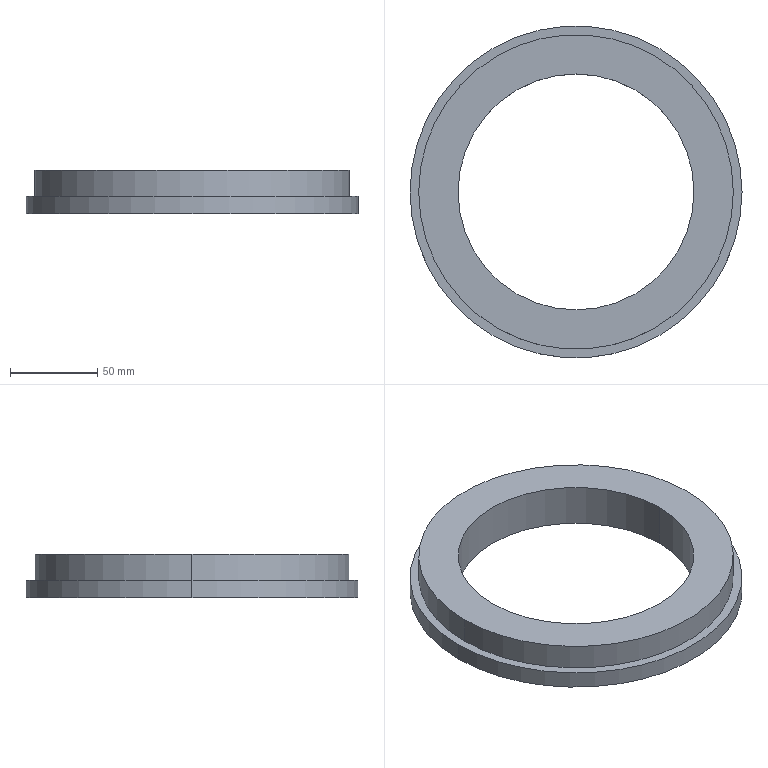Part | SolidWorks | features 3DProfileFeature 1, Extrusion 1, HoleWzd 1, ICE 1 | 1 solid | 33 faces | box 190 x 190 x 25 mm | volume 301982 mm3 | cylinder 18 | cone 12 | plane 3 | commonest cylinder face diameters 10.2 x12 135 x2 180 x2 190 x2
STEP:
#1=CARTESIAN_POINT('',(5.1,80.5,10.));
#2=VERTEX_POINT('',#1);
#3=CARTESIAN_POINT('',(-5.1,80.5,10.));
#4=VERTEX_POINT('',#3);
#5=CARTESIAN_POINT('',(0.,80.5,10.));
#6=DIRECTION('',(0.,0.,-1.));
#7=DIRECTION('',(-1.,0.,0.));
#8=AXIS2_PLACEMENT_3D('',#5,#6,#7);
#9=CIRCLE('',#8,5.1);
#10=EDGE_CURVE('',#2,#4,#9,.T.);
#11=ORIENTED_EDGE('',*,*,#10,.F.);
#12=CARTESIAN_POINT('',(5.1,80.5,0.));
#13=VERTEX_POINT('',#12);
#14=CARTESIAN_POINT('',(5.1,80.5,0.));
#15=DIRECTION('',(0.,0.,-1.));
#16=VECTOR('',#15,1000.);
#17=LINE('',#14,#16);
#18=EDGE_CURVE('',#2,#13,#17,.T.);
#19=ORIENTED_EDGE('',*,*,#18,.T.);
#20=CARTESIAN_POINT('',(-5.1,80.5,0.));
#21=VERTEX_POINT('',#20);
#22=CARTESIAN_POINT('',(0.,80.5,0.));
#23=DIRECTION('',(0.,0.,-1.));
#24=DIRECTION('',(-1.,0.,0.));
#25=AXIS2_PLACEMENT_3D('',#22,#23,#24);
#26=CIRCLE('',#25,5.1);
#27=EDGE_CURVE('',#13,#21,#26,.T.);
#28=ORIENTED_EDGE('',*,*,#27,.T.);
#29=CARTESIAN_POINT('',(-5.1,80.5,0.));
#30=DIRECTION('',(0.,0.,-1.));
#31=VECTOR('',#30,1000.);
#32=LINE('',#29,#31);
#33=EDGE_CURVE('',#4,#21,#32,.T.);
#34=ORIENTED_EDGE('',*,*,#33,.F.);
#35=EDGE_LOOP('',(#11,#19,#28,#34));
#36=FACE_OUTER_BOUND('',#35,.T.);
#37=CARTESIAN_POINT('',(0.,80.5,0.));
#38=DIRECTION('',(0.,0.,-1.));
#39=DIRECTION('',(-1.,0.,0.));
#40=AXIS2_PLACEMENT_3D('',#37,#38,#39);
#41=CYLINDRICAL_SURFACE('',#40,5.1);
#42=ADVANCED_FACE('',(#36),#41,.F.);
#43=CARTESIAN_POINT('',(0.,80.5,13.064));
#44=VERTEX_POINT('',#43);
#45=CARTESIAN_POINT('',(-5.1,80.5,10.));
#46=DIRECTION('',(-0.8572,0.,-0.515));
#47=VECTOR('',#46,1000.);
#48=LINE('',#45,#47);
#49=EDGE_CURVE('',#44,#4,#48,.T.);
#50=ORIENTED_EDGE('',*,*,#49,.F.);
#51=CARTESIAN_POINT('',(5.1,80.5,10.));
#52=DIRECTION('',(0.8572,0.,-0.515));
#53=VECTOR('',#52,1000.);
#54=LINE('',#51,#53);
#55=EDGE_CURVE('',#44,#2,#54,.T.);
#56=ORIENTED_EDGE('',*,*,#55,.T.);
#57=ORIENTED_EDGE('',*,*,#10,.T.);
#58=EDGE_LOOP('',(#50,#56,#57));
#59=FACE_OUTER_BOUND('',#58,.T.);
#60=CARTESIAN_POINT('',(0.,80.5,10.));
#61=DIRECTION('',(0.,0.,-1.));
#62=DIRECTION('',(-1.,0.,0.));
#63=AXIS2_PLACEMENT_3D('',#60,#61,#62);
#64=CONICAL_SURFACE('',#63,5.1,1.03);
#65=ADVANCED_FACE('',(#59),#64,.F.);
#66=CARTESIAN_POINT('',(74.815,40.25,10.));
#67=VERTEX_POINT('',#66);
#68=CARTESIAN_POINT('',(64.615,40.25,10.));
#69=VERTEX_POINT('',#68);
#70=CARTESIAN_POINT('',(69.715,40.25,10.));
#71=DIRECTION('',(0.,0.,-1.));
#72=DIRECTION('',(-1.,0.,0.));
#73=AXIS2_PLACEMENT_3D('',#70,#71,#72);
#74=CIRCLE('',#73,5.1);
#75=EDGE_CURVE('',#67,#69,#74,.T.);
#76=ORIENTED_EDGE('',*,*,#75,.F.);
#77=CARTESIAN_POINT('',(74.815,40.25,0.));
#78=VERTEX_POINT('',#77);
#79=CARTESIAN_POINT('',(74.815,40.25,0.));
#80=DIRECTION('',(0.,0.,-1.));
#81=VECTOR('',#80,1000.);
#82=LINE('',#79,#81);
#83=EDGE_CURVE('',#67,#78,#82,.T.);
#84=ORIENTED_EDGE('',*,*,#83,.T.);
#85=CARTESIAN_POINT('',(64.615,40.25,0.));
#86=VERTEX_POINT('',#85);
#87=CARTESIAN_POINT('',(69.715,40.25,0.));
#88=DIRECTION('',(0.,0.,-1.));
#89=DIRECTION('',(-1.,0.,0.));
#90=AXIS2_PLACEMENT_3D('',#87,#88,#89);
#91=CIRCLE('',#90,5.1);
#92=EDGE_CURVE('',#78,#86,#91,.T.);
#93=ORIENTED_EDGE('',*,*,#92,.T.);
#94=CARTESIAN_POINT('',(64.615,40.25,0.));
#95=DIRECTION('',(0.,0.,-1.));
#96=VECTOR('',#95,1000.);
#97=LINE('',#94,#96);
#98=EDGE_CURVE('',#69,#86,#97,.T.);
#99=ORIENTED_EDGE('',*,*,#98,.F.);
#100=EDGE_LOOP('',(#76,#84,#93,#99));
#101=FACE_OUTER_BOUND('',#100,.T.);
#102=CARTESIAN_POINT('',(69.715,40.25,0.));
#103=DIRECTION('',(0.,0.,-1.));
#104=DIRECTION('',(-1.,0.,0.));
#105=AXIS2_PLACEMENT_3D('',#102,#103,#104);
#106=CYLINDRICAL_SURFACE('',#105,5.1);
#107=ADVANCED_FACE('',(#101),#106,.F.);
#108=CARTESIAN_POINT('',(69.715,40.25,13.064));
#109=VERTEX_POINT('',#108);
#110=CARTESIAN_POINT('',(64.615,40.25,10.));
#111=DIRECTION('',(-0.8572,0.,-0.515));
#112=VECTOR('',#111,1000.);
#113=LINE('',#110,#112);
#114=EDGE_CURVE('',#109,#69,#113,.T.);
#115=ORIENTED_EDGE('',*,*,#114,.F.);
#116=CARTESIAN_POINT('',(74.815,40.25,10.));
#117=DIRECTION('',(0.8572,0.,-0.515));
#118=VECTOR('',#117,1000.);
#119=LINE('',#116,#118);
#120=EDGE_CURVE('',#109,#67,#119,.T.);
#121=ORIENTED_EDGE('',*,*,#120,.T.);
#122=ORIENTED_EDGE('',*,*,#75,.T.);
#123=EDGE_LOOP('',(#115,#121,#122));
#124=FACE_OUTER_BOUND('',#123,.T.);
#125=CARTESIAN_POINT('',(69.715,40.25,10.));
#126=DIRECTION('',(0.,0.,-1.));
#127=DIRECTION('',(-1.,0.,0.));
#128=AXIS2_PLACEMENT_3D('',#125,#126,#127);
#129=CONICAL_SURFACE('',#128,5.1,1.03);
#130=ADVANCED_FACE('',(#124),#129,.F.);
#131=CARTESIAN_POINT('',(74.815,-40.25,10.));
#132=VERTEX_POINT('',#131);
#133=CARTESIAN_POINT('',(64.615,-40.25,10.));
#134=VERTEX_POINT('',#133);
#135=CARTESIAN_POINT('',(69.715,-40.25,10.));
#136=DIRECTION('',(0.,0.,-1.));
#137=DIRECTION('',(-1.,0.,0.));
#138=AXIS2_PLACEMENT_3D('',#135,#136,#137);
#139=CIRCLE('',#138,5.1);
#140=EDGE_CURVE('',#132,#134,#139,.T.);
#141=ORIENTED_EDGE('',*,*,#140,.F.);
#142=CARTESIAN_POINT('',(74.815,-40.25,0.));
#143=VERTEX_POINT('',#142);
#144=CARTESIAN_POINT('',(74.815,-40.25,0.));
#145=DIRECTION('',(0.,0.,-1.));
#146=VECTOR('',#145,1000.);
#147=LINE('',#144,#146);
#148=EDGE_CURVE('',#132,#143,#147,.T.);
#149=ORIENTED_EDGE('',*,*,#148,.T.);
#150=CARTESIAN_POINT('',(64.615,-40.25,0.));
#151=VERTEX_POINT('',#150);
#152=CARTESIAN_POINT('',(69.715,-40.25,0.));
#153=DIRECTION('',(0.,0.,-1.));
#154=DIRECTION('',(-1.,0.,0.));
#155=AXIS2_PLACEMENT_3D('',#152,#153,#154);
#156=CIRCLE('',#155,5.1);
#157=EDGE_CURVE('',#143,#151,#156,.T.);
#158=ORIENTED_EDGE('',*,*,#157,.T.);
#159=CARTESIAN_POINT('',(64.615,-40.25,0.));
#160=DIRECTION('',(0.,0.,-1.));
#161=VECTOR('',#160,1000.);
#162=LINE('',#159,#161);
#163=EDGE_CURVE('',#134,#151,#162,.T.);
#164=ORIENTED_EDGE('',*,*,#163,.F.);
#165=EDGE_LOOP('',(#141,#149,#158,#164));
#166=FACE_OUTER_BOUND('',#165,.T.);
#167=CARTESIAN_POINT('',(69.715,-40.25,0.));
#168=DIRECTION('',(0.,0.,-1.));
#169=DIRECTION('',(-1.,0.,0.));
#170=AXIS2_PLACEMENT_3D('',#167,#168,#169);
#171=CYLINDRICAL_SURFACE('',#170,5.1);
#172=ADVANCED_FACE('',(#166),#171,.F.);
#173=CARTESIAN_POINT('',(69.715,-40.25,13.064));
#174=VERTEX_POINT('',#173);
#175=CARTESIAN_POINT('',(64.615,-40.25,10.));
#176=DIRECTION('',(-0.8572,0.,-0.515));
#177=VECTOR('',#176,1000.);
#178=LINE('',#175,#177);
#179=EDGE_CURVE('',#174,#134,#178,.T.);
#180=ORIENTED_EDGE('',*,*,#179,.F.);
#181=CARTESIAN_POINT('',(74.815,-40.25,10.));
#182=DIRECTION('',(0.8572,0.,-0.515));
#183=VECTOR('',#182,1000.);
#184=LINE('',#181,#183);
#185=EDGE_CURVE('',#174,#132,#184,.T.);
#186=ORIENTED_EDGE('',*,*,#185,.T.);
#187=ORIENTED_EDGE('',*,*,#140,.T.);
#188=EDGE_LOOP('',(#180,#186,#187));
#189=FACE_OUTER_BOUND('',#188,.T.);
#190=CARTESIAN_POINT('',(69.715,-40.25,10.));
#191=DIRECTION('',(0.,0.,-1.));
#192=DIRECTION('',(-1.,0.,0.));
#193=AXIS2_PLACEMENT_3D('',#190,#191,#192);
#194=CONICAL_SURFACE('',#193,5.1,1.03);
#195=ADVANCED_FACE('',(#189),#194,.F.);
#196=CARTESIAN_POINT('',(5.1,-80.5,10.));
#197=VERTEX_POINT('',#196);
#198=CARTESIAN_POINT('',(-5.1,-80.5,10.));
#199=VERTEX_POINT('',#198);
#200=CARTESIAN_POINT('',(0.,-80.5,10.));
#201=DIRECTION('',(0.,0.,-1.));
#202=DIRECTION('',(-1.,0.,0.));
#203=AXIS2_PLACEMENT_3D('',#200,#201,#202);
#204=CIRCLE('',#203,5.1);
#205=EDGE_CURVE('',#197,#199,#204,.T.);
#206=ORIENTED_EDGE('',*,*,#205,.F.);
#207=CARTESIAN_POINT('',(5.1,-80.5,0.));
#208=VERTEX_POINT('',#207);
#209=CARTESIAN_POINT('',(5.1,-80.5,0.));
#210=DIRECTION('',(0.,0.,-1.));
#211=VECTOR('',#210,1000.);
#212=LINE('',#209,#211);
#213=EDGE_CURVE('',#197,#208,#212,.T.);
#214=ORIENTED_EDGE('',*,*,#213,.T.);
#215=CARTESIAN_POINT('',(-5.1,-80.5,0.));
#216=VERTEX_POINT('',#215);
#217=CARTESIAN_POINT('',(0.,-80.5,0.));
#218=DIRECTION('',(0.,0.,-1.));
#219=DIRECTION('',(-1.,0.,0.));
#220=AXIS2_PLACEMENT_3D('',#217,#218,#219);
#221=CIRCLE('',#220,5.1);
#222=EDGE_CURVE('',#208,#216,#221,.T.);
#223=ORIENTED_EDGE('',*,*,#222,.T.);
#224=CARTESIAN_POINT('',(-5.1,-80.5,0.));
#225=DIRECTION('',(0.,0.,-1.));
#226=VECTOR('',#225,1000.);
#227=LINE('',#224,#226);
#228=EDGE_CURVE('',#199,#216,#227,.T.);
#229=ORIENTED_EDGE('',*,*,#228,.F.);
#230=EDGE_LOOP('',(#206,#214,#223,#229));
#231=FACE_OUTER_BOUND('',#230,.T.);
#232=CARTESIAN_POINT('',(0.,-80.5,0.));
#233=DIRECTION('',(0.,0.,-1.));
#234=DIRECTION('',(-1.,0.,0.));
#235=AXIS2_PLACEMENT_3D('',#232,#233,#234);
#236=CYLINDRICAL_SURFACE('',#235,5.1);
#237=ADVANCED_FACE('',(#231),#236,.F.);
#238=CARTESIAN_POINT('',(0.,-80.5,13.064));
#239=VERTEX_POINT('',#238);
#240=CARTESIAN_POINT('',(-5.1,-80.5,10.));
#241=DIRECTION('',(-0.8572,0.,-0.515));
#242=VECTOR('',#241,1000.);
#243=LINE('',#240,#242);
#244=EDGE_CURVE('',#239,#199,#243,.T.);
#245=ORIENTED_EDGE('',*,*,#244,.F.);
#246=CARTESIAN_POINT('',(5.1,-80.5,10.));
#247=DIRECTION('',(0.8572,0.,-0.515));
#248=VECTOR('',#247,1000.);
#249=LINE('',#246,#248);
#250=EDGE_CURVE('',#239,#197,#249,.T.);
#251=ORIENTED_EDGE('',*,*,#250,.T.);
#252=ORIENTED_EDGE('',*,*,#205,.T.);
#253=EDGE_LOOP('',(#245,#251,#252));
#254=FACE_OUTER_BOUND('',#253,.T.);
#255=CARTESIAN_POINT('',(0.,-80.5,10.));
#256=DIRECTION('',(0.,0.,-1.));
#257=DIRECTION('',(-1.,0.,0.));
#258=AXIS2_PLACEMENT_3D('',#255,#256,#257);
#259=CONICAL_SURFACE('',#258,5.1,1.03);
#260=ADVANCED_FACE('',(#254),#259,.F.);
#261=CARTESIAN_POINT('',(-64.615,-40.25,10.));
#262=VERTEX_POINT('',#261);
#263=CARTESIAN_POINT('',(-74.815,-40.25,10.));
#264=VERTEX_POINT('',#263);
#265=CARTESIAN_POINT('',(-69.715,-40.25,10.));
#266=DIRECTION('',(0.,0.,-1.));
#267=DIRECTION('',(-1.,0.,0.));
#268=AXIS2_PLACEMENT_3D('',#265,#266,#267);
#269=CIRCLE('',#268,5.1);
#270=EDGE_CURVE('',#262,#264,#269,.T.);
#271=ORIENTED_EDGE('',*,*,#270,.F.);
#272=CARTESIAN_POINT('',(-64.615,-40.25,0.));
#273=VERTEX_POINT('',#272);
#274=CARTESIAN_POINT('',(-64.615,-40.25,0.));
#275=DIRECTION('',(0.,0.,-1.));
#276=VECTOR('',#275,1000.);
#277=LINE('',#274,#276);
#278=EDGE_CURVE('',#262,#273,#277,.T.);
#279=ORIENTED_EDGE('',*,*,#278,.T.);
#280=CARTESIAN_POINT('',(-74.815,-40.25,0.));
#281=VERTEX_POINT('',#280);
#282=CARTESIAN_POINT('',(-69.715,-40.25,0.));
#283=DIRECTION('',(0.,0.,-1.));
#284=DIRECTION('',(-1.,0.,0.));
#285=AXIS2_PLACEMENT_3D('',#282,#283,#284);
#286=CIRCLE('',#285,5.1);
#287=EDGE_CURVE('',#273,#281,#286,.T.);
#288=ORIENTED_EDGE('',*,*,#287,.T.);
#289=CARTESIAN_POINT('',(-74.815,-40.25,0.));
#290=DIRECTION('',(0.,0.,-1.));
#291=VECTOR('',#290,1000.);
#292=LINE('',#289,#291);
#293=EDGE_CURVE('',#264,#281,#292,.T.);
#294=ORIENTED_EDGE('',*,*,#293,.F.);
#295=EDGE_LOOP('',(#271,#279,#288,#294));
#296=FACE_OUTER_BOUND('',#295,.T.);
#297=CARTESIAN_POINT('',(-69.715,-40.25,0.));
#298=DIRECTION('',(0.,0.,-1.));
#299=DIRECTION('',(-1.,0.,0.));
#300=AXIS2_PLACEMENT_3D('',#297,#298,#299);
#301=CYLINDRICAL_SURFACE('',#300,5.1);
#302=ADVANCED_FACE('',(#296),#301,.F.);
#303=CARTESIAN_POINT('',(-69.715,-40.25,13.064));
#304=VERTEX_POINT('',#303);
#305=CARTESIAN_POINT('',(-74.815,-40.25,10.));
#306=DIRECTION('',(-0.8572,0.,-0.515));
#307=VECTOR('',#306,1000.);
#308=LINE('',#305,#307);
#309=EDGE_CURVE('',#304,#264,#308,.T.);
#310=ORIENTED_EDGE('',*,*,#309,.F.);
#311=CARTESIAN_POINT('',(-64.615,-40.25,10.));
#312=DIRECTION('',(0.8572,0.,-0.515));
#313=VECTOR('',#312,1000.);
#314=LINE('',#311,#313);
#315=EDGE_CURVE('',#304,#262,#314,.T.);
#316=ORIENTED_EDGE('',*,*,#315,.T.);
#317=ORIENTED_EDGE('',*,*,#270,.T.);
#318=EDGE_LOOP('',(#310,#316,#317));
#319=FACE_OUTER_BOUND('',#318,.T.);
#320=CARTESIAN_POINT('',(-69.715,-40.25,10.));
#321=DIRECTION('',(0.,0.,-1.));
#322=DIRECTION('',(-1.,0.,0.));
#323=AXIS2_PLACEMENT_3D('',#320,#321,#322);
#324=CONICAL_SURFACE('',#323,5.1,1.03);
#325=ADVANCED_FACE('',(#319),#324,.F.);
#326=CARTESIAN_POINT('',(-64.615,40.25,10.));
#327=VERTEX_POINT('',#326);
#328=CARTESIAN_POINT('',(-74.815,40.25,10.));
#329=VERTEX_POINT('',#328);
#330=CARTESIAN_POINT('',(-69.715,40.25,10.));
#331=DIRECTION('',(0.,0.,-1.));
#332=DIRECTION('',(-1.,0.,0.));
#333=AXIS2_PLACEMENT_3D('',#330,#331,#332);
#334=CIRCLE('',#333,5.1);
#335=EDGE_CURVE('',#327,#329,#334,.T.);
#336=ORIENTED_EDGE('',*,*,#335,.F.);
#337=CARTESIAN_POINT('',(-64.615,40.25,0.));
#338=VERTEX_POINT('',#337);
#339=CARTESIAN_POINT('',(-64.615,40.25,0.));
#340=DIRECTION('',(0.,0.,-1.));
#341=VECTOR('',#340,1000.);
#342=LINE('',#339,#341);
#343=EDGE_CURVE('',#327,#338,#342,.T.);
#344=ORIENTED_EDGE('',*,*,#343,.T.);
#345=CARTESIAN_POINT('',(-74.815,40.25,0.));
#346=VERTEX_POINT('',#345);
#347=CARTESIAN_POINT('',(-69.715,40.25,0.));
#348=DIRECTION('',(0.,0.,-1.));
#349=DIRECTION('',(-1.,0.,0.));
#350=AXIS2_PLACEMENT_3D('',#347,#348,#349);
#351=CIRCLE('',#350,5.1);
#352=EDGE_CURVE('',#338,#346,#351,.T.);
#353=ORIENTED_EDGE('',*,*,#352,.T.);
#354=CARTESIAN_POINT('',(-74.815,40.25,0.));
#355=DIRECTION('',(0.,0.,-1.));
#356=VECTOR('',#355,1000.);
#357=LINE('',#354,#356);
#358=EDGE_CURVE('',#329,#346,#357,.T.);
#359=ORIENTED_EDGE('',*,*,#358,.F.);
#360=EDGE_LOOP('',(#336,#344,#353,#359));
#361=FACE_OUTER_BOUND('',#360,.T.);
#362=CARTESIAN_POINT('',(-69.715,40.25,0.));
#363=DIRECTION('',(0.,0.,-1.));
#364=DIRECTION('',(-1.,0.,0.));
#365=AXIS2_PLACEMENT_3D('',#362,#363,#364);
#366=CYLINDRICAL_SURFACE('',#365,5.1);
#367=ADVANCED_FACE('',(#361),#366,.F.);
#368=CARTESIAN_POINT('',(-69.715,40.25,13.064));
#369=VERTEX_POINT('',#368);
#370=CARTESIAN_POINT('',(-74.815,40.25,10.));
#371=DIRECTION('',(-0.8572,0.,-0.515));
#372=VECTOR('',#371,1000.);
#373=LINE('',#370,#372);
#374=EDGE_CURVE('',#369,#329,#373,.T.);
#375=ORIENTED_EDGE('',*,*,#374,.F.);
#376=CARTESIAN_POINT('',(-64.615,40.25,10.));
#377=DIRECTION('',(0.8572,0.,-0.515));
#378=VECTOR('',#377,1000.);
#379=LINE('',#376,#378);
#380=EDGE_CURVE('',#369,#327,#379,.T.);
#381=ORIENTED_EDGE('',*,*,#380,.T.);
#382=ORIENTED_EDGE('',*,*,#335,.T.);
#383=EDGE_LOOP('',(#375,#381,#382));
#384=FACE_OUTER_BOUND('',#383,.T.);
#385=CARTESIAN_POINT('',(-69.715,40.25,10.));
#386=DIRECTION('',(0.,0.,-1.));
#387=DIRECTION('',(-1.,0.,0.));
#388=AXIS2_PLACEMENT_3D('',#385,#386,#387);
#389=CONICAL_SURFACE('',#388,5.1,1.03);
#390=ADVANCED_FACE('',(#384),#389,.F.);
#391=CARTESIAN_POINT('',(90.,0.,25.));
#392=VERTEX_POINT('',#391);
#393=CARTESIAN_POINT('',(-90.,0.,25.));
#394=VERTEX_POINT('',#393);
#395=CARTESIAN_POINT('',(0.,0.,25.));
#396=DIRECTION('',(0.,0.,1.));
#397=DIRECTION('',(1.,0.,0.));
#398=AXIS2_PLACEMENT_3D('',#395,#396,#397);
#399=CIRCLE('',#398,90.);
#400=EDGE_CURVE('',#392,#394,#399,.T.);
#401=ORIENTED_EDGE('',*,*,#400,.F.);
#402=CARTESIAN_POINT('',(90.,0.,10.));
#403=VERTEX_POINT('',#402);
#404=CARTESIAN_POINT('',(90.,0.,25.));
#405=DIRECTION('',(0.,0.,-1.));
#406=VECTOR('',#405,1000.);
#407=LINE('',#404,#406);
#408=EDGE_CURVE('',#392,#403,#407,.T.);
#409=ORIENTED_EDGE('',*,*,#408,.T.);
#410=CARTESIAN_POINT('',(-90.,0.,10.));
#411=VERTEX_POINT('',#410);
#412=CARTESIAN_POINT('',(0.,0.,10.));
#413=DIRECTION('',(0.,0.,1.));
#414=DIRECTION('',(1.,0.,0.));
#415=AXIS2_PLACEMENT_3D('',#412,#413,#414);
#416=CIRCLE('',#415,90.);
#417=EDGE_CURVE('',#403,#411,#416,.T.);
#418=ORIENTED_EDGE('',*,*,#417,.T.);
#419=CARTESIAN_POINT('',(-90.,0.,25.));
#420=DIRECTION('',(0.,0.,-1.));
#421=VECTOR('',#420,1000.);
#422=LINE('',#419,#421);
#423=EDGE_CURVE('',#394,#411,#422,.T.);
#424=ORIENTED_EDGE('',*,*,#423,.F.);
#425=EDGE_LOOP('',(#401,#409,#418,#424));
#426=FACE_OUTER_BOUND('',#425,.T.);
#427=CARTESIAN_POINT('',(0.,0.,25.));
#428=DIRECTION('',(0.,0.,-1.));
#429=DIRECTION('',(-1.,0.,0.));
#430=AXIS2_PLACEMENT_3D('',#427,#428,#429);
#431=CYLINDRICAL_SURFACE('',#430,90.);
#432=ADVANCED_FACE('',(#426),#431,.T.);
#433=CARTESIAN_POINT('',(-67.5,0.,25.));
#434=VERTEX_POINT('',#433);
#435=CARTESIAN_POINT('',(67.5,0.,25.));
#436=VERTEX_POINT('',#435);
#437=CARTESIAN_POINT('',(0.,0.,25.));
#438=DIRECTION('',(0.,0.,1.));
#439=DIRECTION('',(1.,0.,0.));
#440=AXIS2_PLACEMENT_3D('',#437,#438,#439);
#441=CIRCLE('',#440,67.5);
#442=EDGE_CURVE('',#434,#436,#441,.T.);
#443=ORIENTED_EDGE('',*,*,#442,.T.);
#444=CARTESIAN_POINT('',(67.5,0.,0.));
#445=VERTEX_POINT('',#444);
#446=CARTESIAN_POINT('',(67.5,0.,10.));
#447=DIRECTION('',(0.,0.,-1.));
#448=VECTOR('',#447,1000.);
#449=LINE('',#446,#448);
#450=EDGE_CURVE('',#436,#445,#449,.T.);
#451=ORIENTED_EDGE('',*,*,#450,.T.);
#452=CARTESIAN_POINT('',(-67.5,0.,0.));
#453=VERTEX_POINT('',#452);
#454=CARTESIAN_POINT('',(0.,0.,0.));
#455=DIRECTION('',(0.,0.,1.));
#456=DIRECTION('',(1.,0.,0.));
#457=AXIS2_PLACEMENT_3D('',#454,#455,#456);
#458=CIRCLE('',#457,67.5);
#459=EDGE_CURVE('',#453,#445,#458,.T.);
#460=ORIENTED_EDGE('',*,*,#459,.F.);
#461=CARTESIAN_POINT('',(-67.5,0.,10.));
#462=DIRECTION('',(0.,0.,-1.));
#463=VECTOR('',#462,1000.);
#464=LINE('',#461,#463);
#465=EDGE_CURVE('',#434,#453,#464,.T.);
#466=ORIENTED_EDGE('',*,*,#465,.F.);
#467=EDGE_LOOP('',(#443,#451,#460,#466));
#468=FACE_OUTER_BOUND('',#467,.T.);
#469=CARTESIAN_POINT('',(0.,0.,10.));
#470=DIRECTION('',(0.,0.,-1.));
#471=DIRECTION('',(-1.,0.,0.));
#472=AXIS2_PLACEMENT_3D('',#469,#470,#471);
#473=CYLINDRICAL_SURFACE('',#472,67.5);
#474=ADVANCED_FACE('',(#468),#473,.F.);
#475=CARTESIAN_POINT('',(95.,0.,10.));
#476=VERTEX_POINT('',#475);
#477=CARTESIAN_POINT('',(-95.,0.,10.));
#478=VERTEX_POINT('',#477);
#479=CARTESIAN_POINT('',(0.,0.,10.));
#480=DIRECTION('',(0.,0.,1.));
#481=DIRECTION('',(1.,0.,0.));
#482=AXIS2_PLACEMENT_3D('',#479,#480,#481);
#483=CIRCLE('',#482,95.);
#484=EDGE_CURVE('',#476,#478,#483,.T.);
#485=ORIENTED_EDGE('',*,*,#484,.F.);
#486=CARTESIAN_POINT('',(95.,0.,0.));
#487=VERTEX_POINT('',#486);
#488=CARTESIAN_POINT('',(95.,0.,10.));
#489=DIRECTION('',(0.,0.,-1.));
#490=VECTOR('',#489,1000.);
#491=LINE('',#488,#490);
#492=EDGE_CURVE('',#476,#487,#491,.T.);
#493=ORIENTED_EDGE('',*,*,#492,.T.);
#494=CARTESIAN_POINT('',(-95.,0.,0.));
#495=VERTEX_POINT('',#494);
#496=CARTESIAN_POINT('',(0.,0.,0.));
#497=DIRECTION('',(0.,0.,1.));
#498=DIRECTION('',(1.,0.,0.));
#499=AXIS2_PLACEMENT_3D('',#496,#497,#498);
#500=CIRCLE('',#499,95.);
#501=EDGE_CURVE('',#487,#495,#500,.T.);
#502=ORIENTED_EDGE('',*,*,#501,.T.);
#503=CARTESIAN_POINT('',(-95.,0.,10.));
#504=DIRECTION('',(0.,0.,-1.));
#505=VECTOR('',#504,1000.);
#506=LINE('',#503,#505);
#507=EDGE_CURVE('',#478,#495,#506,.T.);
#508=ORIENTED_EDGE('',*,*,#507,.F.);
#509=EDGE_LOOP('',(#485,#493,#502,#508));
#510=FACE_OUTER_BOUND('',#509,.T.);
#511=CARTESIAN_POINT('',(0.,0.,10.));
#512=DIRECTION('',(0.,0.,-1.));
#513=DIRECTION('',(-1.,0.,0.));
#514=AXIS2_PLACEMENT_3D('',#511,#512,#513);
#515=CYLINDRICAL_SURFACE('',#514,95.);
#516=ADVANCED_FACE('',(#510),#515,.T.);
#517=CARTESIAN_POINT('',(0.,0.,10.));
#518=DIRECTION('',(0.,0.,1.));
#519=DIRECTION('',(1.,0.,0.));
#520=AXIS2_PLACEMENT_3D('',#517,#518,#519);
#521=CIRCLE('',#520,95.);
#522=EDGE_CURVE('',#478,#476,#521,.T.);
#523=ORIENTED_EDGE('',*,*,#522,.T.);
#524=ORIENTED_EDGE('',*,*,#484,.T.);
#525=EDGE_LOOP('',(#523,#524));
#526=FACE_OUTER_BOUND('',#525,.T.);
#527=CARTESIAN_POINT('',(0.,0.,10.));
#528=DIRECTION('',(0.,0.,1.));
#529=DIRECTION('',(1.,0.,0.));
#530=AXIS2_PLACEMENT_3D('',#527,#528,#529);
#531=CIRCLE('',#530,90.);
#532=EDGE_CURVE('',#411,#403,#531,.T.);
#533=ORIENTED_EDGE('',*,*,#532,.F.);
#534=ORIENTED_EDGE('',*,*,#417,.F.);
#535=EDGE_LOOP('',(#533,#534));
#536=FACE_BOUND('',#535,.T.);
#537=CARTESIAN_POINT('',(0.,0.,10.));
#538=DIRECTION('',(0.,0.,1.));
#539=DIRECTION('',(1.,0.,0.));
#540=AXIS2_PLACEMENT_3D('',#537,#538,#539);
#541=PLANE('',#540);
#542=ADVANCED_FACE('',(#526,#536),#541,.T.);
#543=CARTESIAN_POINT('',(0.,80.5,0.));
#544=DIRECTION('',(0.,0.,-1.));
#545=DIRECTION('',(-1.,0.,0.));
#546=AXIS2_PLACEMENT_3D('',#543,#544,#545);
#547=CIRCLE('',#546,5.1);
#548=EDGE_CURVE('',#21,#13,#547,.T.);
#549=ORIENTED_EDGE('',*,*,#548,.F.);
#550=ORIENTED_EDGE('',*,*,#27,.F.);
#551=EDGE_LOOP('',(#549,#550));
#552=FACE_BOUND('',#551,.T.);
#553=CARTESIAN_POINT('',(69.715,40.25,0.));
#554=DIRECTION('',(0.,0.,-1.));
#555=DIRECTION('',(-1.,0.,0.));
#556=AXIS2_PLACEMENT_3D('',#553,#554,#555);
#557=CIRCLE('',#556,5.1);
#558=EDGE_CURVE('',#86,#78,#557,.T.);
#559=ORIENTED_EDGE('',*,*,#558,.F.);
#560=ORIENTED_EDGE('',*,*,#92,.F.);
#561=EDGE_LOOP('',(#559,#560));
#562=FACE_BOUND('',#561,.T.);
#563=CARTESIAN_POINT('',(69.715,-40.25,0.));
#564=DIRECTION('',(0.,0.,-1.));
#565=DIRECTION('',(-1.,0.,0.));
#566=AXIS2_PLACEMENT_3D('',#563,#564,#565);
#567=CIRCLE('',#566,5.1);
#568=EDGE_CURVE('',#151,#143,#567,.T.);
#569=ORIENTED_EDGE('',*,*,#568,.F.);
#570=ORIENTED_EDGE('',*,*,#157,.F.);
#571=EDGE_LOOP('',(#569,#570));
#572=FACE_BOUND('',#571,.T.);
#573=CARTESIAN_POINT('',(0.,-80.5,0.));
#574=DIRECTION('',(0.,0.,-1.));
#575=DIRECTION('',(-1.,0.,0.));
#576=AXIS2_PLACEMENT_3D('',#573,#574,#575);
#577=CIRCLE('',#576,5.1);
#578=EDGE_CURVE('',#216,#208,#577,.T.);
#579=ORIENTED_EDGE('',*,*,#578,.F.);
#580=ORIENTED_EDGE('',*,*,#222,.F.);
#581=EDGE_LOOP('',(#579,#580));
#582=FACE_BOUND('',#581,.T.);
#583=CARTESIAN_POINT('',(-69.715,-40.25,0.));
#584=DIRECTION('',(0.,0.,-1.));
#585=DIRECTION('',(-1.,0.,0.));
#586=AXIS2_PLACEMENT_3D('',#583,#584,#585);
#587=CIRCLE('',#586,5.1);
#588=EDGE_CURVE('',#281,#273,#587,.T.);
#589=ORIENTED_EDGE('',*,*,#588,.F.);
#590=ORIENTED_EDGE('',*,*,#287,.F.);
#591=EDGE_LOOP('',(#589,#590));
#592=FACE_BOUND('',#591,.T.);
#593=CARTESIAN_POINT('',(-69.715,40.25,0.));
#594=DIRECTION('',(0.,0.,-1.));
#595=DIRECTION('',(-1.,0.,0.));
#596=AXIS2_PLACEMENT_3D('',#593,#594,#595);
#597=CIRCLE('',#596,5.1);
#598=EDGE_CURVE('',#346,#338,#597,.T.);
#599=ORIENTED_EDGE('',*,*,#598,.F.);
#600=ORIENTED_EDGE('',*,*,#352,.F.);
#601=EDGE_LOOP('',(#599,#600));
#602=FACE_BOUND('',#601,.T.);
#603=CARTESIAN_POINT('',(0.,0.,0.));
#604=DIRECTION('',(0.,0.,1.));
#605=DIRECTION('',(1.,0.,0.));
#606=AXIS2_PLACEMENT_3D('',#603,#604,#605);
#607=CIRCLE('',#606,95.);
#608=EDGE_CURVE('',#495,#487,#607,.T.);
#609=ORIENTED_EDGE('',*,*,#608,.F.);
#610=ORIENTED_EDGE('',*,*,#501,.F.);
#611=EDGE_LOOP('',(#609,#610));
#612=FACE_OUTER_BOUND('',#611,.T.);
#613=ORIENTED_EDGE('',*,*,#459,.T.);
#614=CARTESIAN_POINT('',(0.,0.,0.));
#615=DIRECTION('',(0.,0.,1.));
#616=DIRECTION('',(1.,0.,0.));
#617=AXIS2_PLACEMENT_3D('',#614,#615,#616);
#618=CIRCLE('',#617,67.5);
#619=EDGE_CURVE('',#445,#453,#618,.T.);
#620=ORIENTED_EDGE('',*,*,#619,.T.);
#621=EDGE_LOOP('',(#613,#620));
#622=FACE_BOUND('',#621,.T.);
#623=CARTESIAN_POINT('',(0.,0.,0.));
#624=DIRECTION('',(0.,0.,1.));
#625=DIRECTION('',(1.,0.,0.));
#626=AXIS2_PLACEMENT_3D('',#623,#624,#625);
#627=PLANE('',#626);
#628=ADVANCED_FACE('',(#552,#562,#572,#582,#592,#602,#612,#622),#627,.F.);
#629=ORIENTED_EDGE('',*,*,#492,.F.);
#630=ORIENTED_EDGE('',*,*,#522,.F.);
#631=ORIENTED_EDGE('',*,*,#507,.T.);
#632=ORIENTED_EDGE('',*,*,#608,.T.);
#633=EDGE_LOOP('',(#629,#630,#631,#632));
#634=FACE_OUTER_BOUND('',#633,.T.);
#635=CARTESIAN_POINT('',(0.,0.,10.));
#636=DIRECTION('',(0.,0.,-1.));
#637=DIRECTION('',(-1.,0.,0.));
#638=AXIS2_PLACEMENT_3D('',#635,#636,#637);
#639=CYLINDRICAL_SURFACE('',#638,95.);
#640=ADVANCED_FACE('',(#634),#639,.T.);
#641=ORIENTED_EDGE('',*,*,#450,.F.);
#642=CARTESIAN_POINT('',(0.,0.,25.));
#643=DIRECTION('',(0.,0.,1.));
#644=DIRECTION('',(1.,0.,0.));
#645=AXIS2_PLACEMENT_3D('',#642,#643,#644);
#646=CIRCLE('',#645,67.5);
#647=EDGE_CURVE('',#436,#434,#646,.T.);
#648=ORIENTED_EDGE('',*,*,#647,.T.);
#649=ORIENTED_EDGE('',*,*,#465,.T.);
#650=ORIENTED_EDGE('',*,*,#619,.F.);
#651=EDGE_LOOP('',(#641,#648,#649,#650));
#652=FACE_OUTER_BOUND('',#651,.T.);
#653=CARTESIAN_POINT('',(0.,0.,10.));
#654=DIRECTION('',(0.,0.,-1.));
#655=DIRECTION('',(-1.,0.,0.));
#656=AXIS2_PLACEMENT_3D('',#653,#654,#655);
#657=CYLINDRICAL_SURFACE('',#656,67.5);
#658=ADVANCED_FACE('',(#652),#657,.F.);
#659=CARTESIAN_POINT('',(0.,0.,25.));
#660=DIRECTION('',(0.,0.,1.));
#661=DIRECTION('',(1.,0.,0.));
#662=AXIS2_PLACEMENT_3D('',#659,#660,#661);
#663=CIRCLE('',#662,90.);
#664=EDGE_CURVE('',#394,#392,#663,.T.);
#665=ORIENTED_EDGE('',*,*,#664,.T.);
#666=ORIENTED_EDGE('',*,*,#400,.T.);
#667=EDGE_LOOP('',(#665,#666));
#668=FACE_OUTER_BOUND('',#667,.T.);
#669=ORIENTED_EDGE('',*,*,#442,.F.);
#670=ORIENTED_EDGE('',*,*,#647,.F.);
#671=EDGE_LOOP('',(#669,#670));
#672=FACE_BOUND('',#671,.T.);
#673=CARTESIAN_POINT('',(0.,0.,25.));
#674=DIRECTION('',(0.,0.,1.));
#675=DIRECTION('',(1.,0.,0.));
#676=AXIS2_PLACEMENT_3D('',#673,#674,#675);
#677=PLANE('',#676);
#678=ADVANCED_FACE('',(#668,#672),#677,.T.);
#679=ORIENTED_EDGE('',*,*,#408,.F.);
#680=ORIENTED_EDGE('',*,*,#664,.F.);
#681=ORIENTED_EDGE('',*,*,#423,.T.);
#682=ORIENTED_EDGE('',*,*,#532,.T.);
#683=EDGE_LOOP('',(#679,#680,#681,#682));
#684=FACE_OUTER_BOUND('',#683,.T.);
#685=CARTESIAN_POINT('',(0.,0.,25.));
#686=DIRECTION('',(0.,0.,-1.));
#687=DIRECTION('',(-1.,0.,0.));
#688=AXIS2_PLACEMENT_3D('',#685,#686,#687);
#689=CYLINDRICAL_SURFACE('',#688,90.);
#690=ADVANCED_FACE('',(#684),#689,.T.);
#691=ORIENTED_EDGE('',*,*,#380,.F.);
#692=ORIENTED_EDGE('',*,*,#374,.T.);
#693=CARTESIAN_POINT('',(-69.715,40.25,10.));
#694=DIRECTION('',(0.,0.,-1.));
#695=DIRECTION('',(-1.,0.,0.));
#696=AXIS2_PLACEMENT_3D('',#693,#694,#695);
#697=CIRCLE('',#696,5.1);
#698=EDGE_CURVE('',#329,#327,#697,.T.);
#699=ORIENTED_EDGE('',*,*,#698,.T.);
#700=EDGE_LOOP('',(#691,#692,#699));
#701=FACE_OUTER_BOUND('',#700,.T.);
#702=CARTESIAN_POINT('',(-69.715,40.25,10.));
#703=DIRECTION('',(0.,0.,-1.));
#704=DIRECTION('',(-1.,0.,0.));
#705=AXIS2_PLACEMENT_3D('',#702,#703,#704);
#706=CONICAL_SURFACE('',#705,5.1,1.03);
#707=ADVANCED_FACE('',(#701),#706,.F.);
#708=ORIENTED_EDGE('',*,*,#343,.F.);
#709=ORIENTED_EDGE('',*,*,#698,.F.);
#710=ORIENTED_EDGE('',*,*,#358,.T.);
#711=ORIENTED_EDGE('',*,*,#598,.T.);
#712=EDGE_LOOP('',(#708,#709,#710,#711));
#713=FACE_OUTER_BOUND('',#712,.T.);
#714=CARTESIAN_POINT('',(-69.715,40.25,0.));
#715=DIRECTION('',(0.,0.,-1.));
#716=DIRECTION('',(-1.,0.,0.));
#717=AXIS2_PLACEMENT_3D('',#714,#715,#716);
#718=CYLINDRICAL_SURFACE('',#717,5.1);
#719=ADVANCED_FACE('',(#713),#718,.F.);
#720=ORIENTED_EDGE('',*,*,#315,.F.);
#721=ORIENTED_EDGE('',*,*,#309,.T.);
#722=CARTESIAN_POINT('',(-69.715,-40.25,10.));
#723=DIRECTION('',(0.,0.,-1.));
#724=DIRECTION('',(-1.,0.,0.));
#725=AXIS2_PLACEMENT_3D('',#722,#723,#724);
#726=CIRCLE('',#725,5.1);
#727=EDGE_CURVE('',#264,#262,#726,.T.);
#728=ORIENTED_EDGE('',*,*,#727,.T.);
#729=EDGE_LOOP('',(#720,#721,#728));
#730=FACE_OUTER_BOUND('',#729,.T.);
#731=CARTESIAN_POINT('',(-69.715,-40.25,10.));
#732=DIRECTION('',(0.,0.,-1.));
#733=DIRECTION('',(-1.,0.,0.));
#734=AXIS2_PLACEMENT_3D('',#731,#732,#733);
#735=CONICAL_SURFACE('',#734,5.1,1.03);
#736=ADVANCED_FACE('',(#730),#735,.F.);
#737=ORIENTED_EDGE('',*,*,#278,.F.);
#738=ORIENTED_EDGE('',*,*,#727,.F.);
#739=ORIENTED_EDGE('',*,*,#293,.T.);
#740=ORIENTED_EDGE('',*,*,#588,.T.);
#741=EDGE_LOOP('',(#737,#738,#739,#740));
#742=FACE_OUTER_BOUND('',#741,.T.);
#743=CARTESIAN_POINT('',(-69.715,-40.25,0.));
#744=DIRECTION('',(0.,0.,-1.));
#745=DIRECTION('',(-1.,0.,0.));
#746=AXIS2_PLACEMENT_3D('',#743,#744,#745);
#747=CYLINDRICAL_SURFACE('',#746,5.1);
#748=ADVANCED_FACE('',(#742),#747,.F.);
#749=ORIENTED_EDGE('',*,*,#250,.F.);
#750=ORIENTED_EDGE('',*,*,#244,.T.);
#751=CARTESIAN_POINT('',(0.,-80.5,10.));
#752=DIRECTION('',(0.,0.,-1.));
#753=DIRECTION('',(-1.,0.,0.));
#754=AXIS2_PLACEMENT_3D('',#751,#752,#753);
#755=CIRCLE('',#754,5.1);
#756=EDGE_CURVE('',#199,#197,#755,.T.);
#757=ORIENTED_EDGE('',*,*,#756,.T.);
#758=EDGE_LOOP('',(#749,#750,#757));
#759=FACE_OUTER_BOUND('',#758,.T.);
#760=CARTESIAN_POINT('',(0.,-80.5,10.));
#761=DIRECTION('',(0.,0.,-1.));
#762=DIRECTION('',(-1.,0.,0.));
#763=AXIS2_PLACEMENT_3D('',#760,#761,#762);
#764=CONICAL_SURFACE('',#763,5.1,1.03);
#765=ADVANCED_FACE('',(#759),#764,.F.);
#766=ORIENTED_EDGE('',*,*,#213,.F.);
#767=ORIENTED_EDGE('',*,*,#756,.F.);
#768=ORIENTED_EDGE('',*,*,#228,.T.);
#769=ORIENTED_EDGE('',*,*,#578,.T.);
#770=EDGE_LOOP('',(#766,#767,#768,#769));
#771=FACE_OUTER_BOUND('',#770,.T.);
#772=CARTESIAN_POINT('',(0.,-80.5,0.));
#773=DIRECTION('',(0.,0.,-1.));
#774=DIRECTION('',(-1.,0.,0.));
#775=AXIS2_PLACEMENT_3D('',#772,#773,#774);
#776=CYLINDRICAL_SURFACE('',#775,5.1);
#777=ADVANCED_FACE('',(#771),#776,.F.);
#778=ORIENTED_EDGE('',*,*,#185,.F.);
#779=ORIENTED_EDGE('',*,*,#179,.T.);
#780=CARTESIAN_POINT('',(69.715,-40.25,10.));
#781=DIRECTION('',(0.,0.,-1.));
#782=DIRECTION('',(-1.,0.,0.));
#783=AXIS2_PLACEMENT_3D('',#780,#781,#782);
#784=CIRCLE('',#783,5.1);
#785=EDGE_CURVE('',#134,#132,#784,.T.);
#786=ORIENTED_EDGE('',*,*,#785,.T.);
#787=EDGE_LOOP('',(#778,#779,#786));
#788=FACE_OUTER_BOUND('',#787,.T.);
#789=CARTESIAN_POINT('',(69.715,-40.25,10.));
#790=DIRECTION('',(0.,0.,-1.));
#791=DIRECTION('',(-1.,0.,0.));
#792=AXIS2_PLACEMENT_3D('',#789,#790,#791);
#793=CONICAL_SURFACE('',#792,5.1,1.03);
#794=ADVANCED_FACE('',(#788),#793,.F.);
#795=ORIENTED_EDGE('',*,*,#148,.F.);
#796=ORIENTED_EDGE('',*,*,#785,.F.);
#797=ORIENTED_EDGE('',*,*,#163,.T.);
#798=ORIENTED_EDGE('',*,*,#568,.T.);
#799=EDGE_LOOP('',(#795,#796,#797,#798));
#800=FACE_OUTER_BOUND('',#799,.T.);
#801=CARTESIAN_POINT('',(69.715,-40.25,0.));
#802=DIRECTION('',(0.,0.,-1.));
#803=DIRECTION('',(-1.,0.,0.));
#804=AXIS2_PLACEMENT_3D('',#801,#802,#803);
#805=CYLINDRICAL_SURFACE('',#804,5.1);
#806=ADVANCED_FACE('',(#800),#805,.F.);
#807=ORIENTED_EDGE('',*,*,#120,.F.);
#808=ORIENTED_EDGE('',*,*,#114,.T.);
#809=CARTESIAN_POINT('',(69.715,40.25,10.));
#810=DIRECTION('',(0.,0.,-1.));
#811=DIRECTION('',(-1.,0.,0.));
#812=AXIS2_PLACEMENT_3D('',#809,#810,#811);
#813=CIRCLE('',#812,5.1);
#814=EDGE_CURVE('',#69,#67,#813,.T.);
#815=ORIENTED_EDGE('',*,*,#814,.T.);
#816=EDGE_LOOP('',(#807,#808,#815));
#817=FACE_OUTER_BOUND('',#816,.T.);
#818=CARTESIAN_POINT('',(69.715,40.25,10.));
#819=DIRECTION('',(0.,0.,-1.));
#820=DIRECTION('',(-1.,0.,0.));
#821=AXIS2_PLACEMENT_3D('',#818,#819,#820);
#822=CONICAL_SURFACE('',#821,5.1,1.03);
#823=ADVANCED_FACE('',(#817),#822,.F.);
#824=ORIENTED_EDGE('',*,*,#83,.F.);
#825=ORIENTED_EDGE('',*,*,#814,.F.);
#826=ORIENTED_EDGE('',*,*,#98,.T.);
#827=ORIENTED_EDGE('',*,*,#558,.T.);
#828=EDGE_LOOP('',(#824,#825,#826,#827));
#829=FACE_OUTER_BOUND('',#828,.T.);
#830=CARTESIAN_POINT('',(69.715,40.25,0.));
#831=DIRECTION('',(0.,0.,-1.));
#832=DIRECTION('',(-1.,0.,0.));
#833=AXIS2_PLACEMENT_3D('',#830,#831,#832);
#834=CYLINDRICAL_SURFACE('',#833,5.1);
#835=ADVANCED_FACE('',(#829),#834,.F.);
#836=ORIENTED_EDGE('',*,*,#55,.F.);
#837=ORIENTED_EDGE('',*,*,#49,.T.);
#838=CARTESIAN_POINT('',(0.,80.5,10.));
#839=DIRECTION('',(0.,0.,-1.));
#840=DIRECTION('',(-1.,0.,0.));
#841=AXIS2_PLACEMENT_3D('',#838,#839,#840);
#842=CIRCLE('',#841,5.1);
#843=EDGE_CURVE('',#4,#2,#842,.T.);
#844=ORIENTED_EDGE('',*,*,#843,.T.);
#845=EDGE_LOOP('',(#836,#837,#844));
#846=FACE_OUTER_BOUND('',#845,.T.);
#847=CARTESIAN_POINT('',(0.,80.5,10.));
#848=DIRECTION('',(0.,0.,-1.));
#849=DIRECTION('',(-1.,0.,0.));
#850=AXIS2_PLACEMENT_3D('',#847,#848,#849);
#851=CONICAL_SURFACE('',#850,5.1,1.03);
#852=ADVANCED_FACE('',(#846),#851,.F.);
#853=ORIENTED_EDGE('',*,*,#18,.F.);
#854=ORIENTED_EDGE('',*,*,#843,.F.);
#855=ORIENTED_EDGE('',*,*,#33,.T.);
#856=ORIENTED_EDGE('',*,*,#548,.T.);
#857=EDGE_LOOP('',(#853,#854,#855,#856));
#858=FACE_OUTER_BOUND('',#857,.T.);
#859=CARTESIAN_POINT('',(0.,80.5,0.));
#860=DIRECTION('',(0.,0.,-1.));
#861=DIRECTION('',(-1.,0.,0.));
#862=AXIS2_PLACEMENT_3D('',#859,#860,#861);
#863=CYLINDRICAL_SURFACE('',#862,5.1);
#864=ADVANCED_FACE('',(#858),#863,.F.);
#865=CLOSED_SHELL('',(#42,#65,#107,#130,#172,#195,#237,#260,#302,#325,#367,#390,#432,#474,#516,#542,#628,#640,#658,#678,#690,#707,#719,#736,#748,#765,#777,#794,#806,#823,#835,#852,#864));
#866=MANIFOLD_SOLID_BREP('',#865);
#867=CARTESIAN_POINT('',(0.,0.,0.));
#868=DIRECTION('',(0.,0.,1.));
#869=DIRECTION('',(1.,0.,0.));
#870=AXIS2_PLACEMENT_3D('',#867,#868,#869);
#871=(LENGTH_UNIT()NAMED_UNIT(*)SI_UNIT(.MILLI.,.METRE.));
#872=UNCERTAINTY_MEASURE_WITH_UNIT(LENGTH_MEASURE(0.00001),#871,'','');
#873=(NAMED_UNIT(*)PLANE_ANGLE_UNIT()SI_UNIT($,.RADIAN.));
#874=(NAMED_UNIT(*)SI_UNIT($,.STERADIAN.)SOLID_ANGLE_UNIT());
#875=(GEOMETRIC_REPRESENTATION_CONTEXT(3)GLOBAL_UNCERTAINTY_ASSIGNED_CONTEXT((#872))GLOBAL_UNIT_ASSIGNED_CONTEXT((#871,#873,#874))REPRESENTATION_CONTEXT('',''));
#876=ADVANCED_BREP_SHAPE_REPRESENTATION('',(#866,#870),#875);